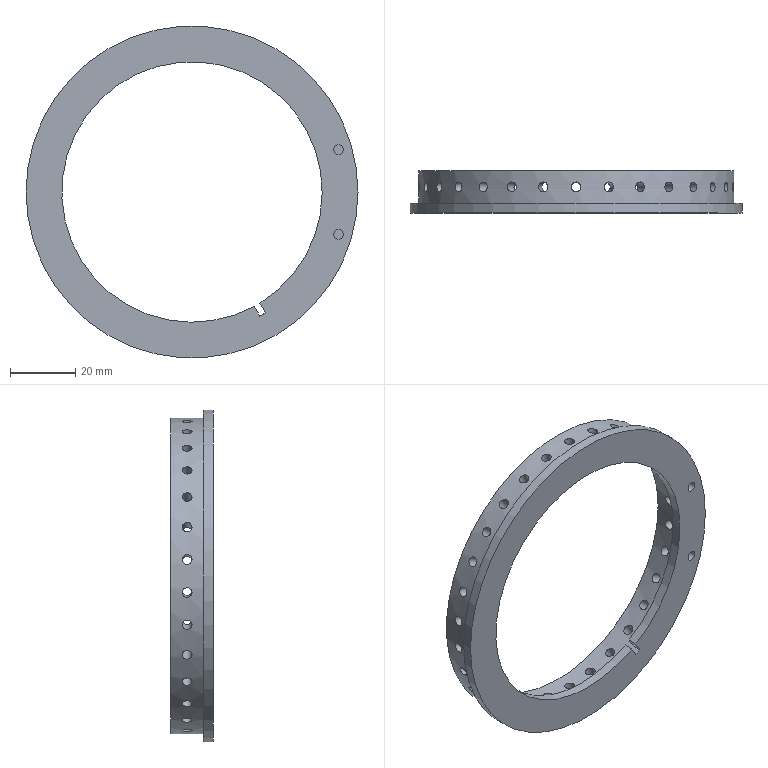Part | STEP file | 1-56.1 | 1 solid | 44 faces | box 102 x 13 x 102 mm | volume 22776 mm3 | cylinder 36 | plane 8 | commonest cylinder face diameters 3 x32 80 x1 87 x1 97 x1 102 x1